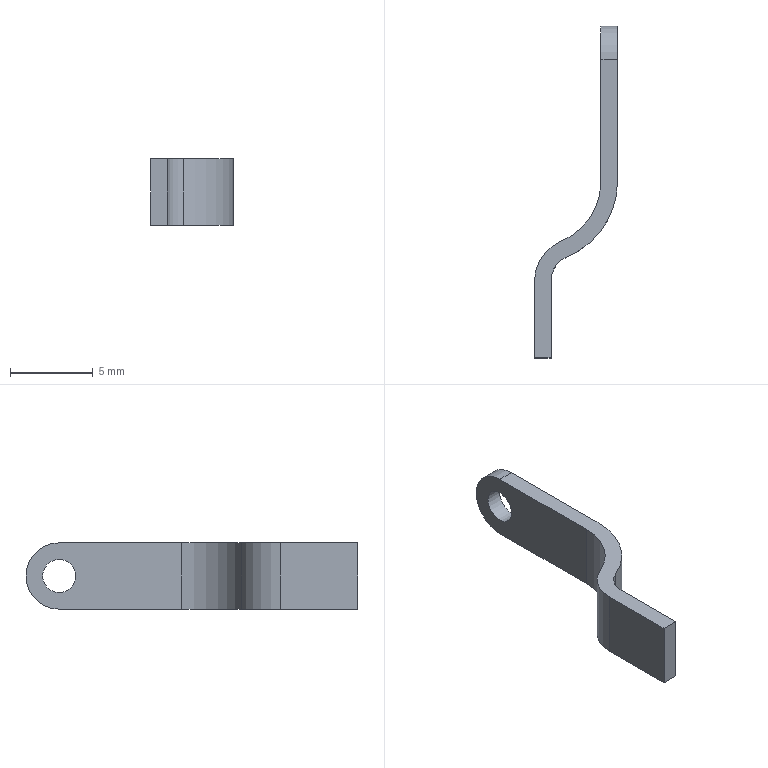Part | STEP file | 1-63.5 | 1 solid | 14 faces | box 5 x 20 x 4 mm | volume 81.74 mm3 | plane 7 | cylinder 7 | commonest cylinder face diameters 4 x2 2 x1 3.13 x1 5.13 x1 7.8 x1 9.8 x1
STEP:
#1=CARTESIAN_POINT('',(0.,0.,0.));
#2=DIRECTION('',(0.,0.,1.));
#3=DIRECTION('',(1.,0.,0.));
#4=AXIS2_PLACEMENT_3D('',#1,#2,#3);
#5=CARTESIAN_POINT('',(-4.,-15.,2.));
#6=VERTEX_POINT('',#5);
#7=CARTESIAN_POINT('',(-4.,-10.352,2.));
#8=VERTEX_POINT('',#7);
#9=CARTESIAN_POINT('',(-4.,-15.,2.));
#10=DIRECTION('',(0.,1.,0.));
#11=VECTOR('',#10,1.);
#12=LINE('',#9,#11);
#13=CARTESIAN_POINT('',(-4.,-12.676,0.));
#14=DIRECTION('',(-1.,0.,0.));
#15=DIRECTION('',(0.,1.,0.));
#16=AXIS2_PLACEMENT_3D('',#13,#14,#15);
#17=PLANE('',#16);
#18=CARTESIAN_POINT('',(-2.324,-2.));
#19=DIRECTION('',(1.,0.));
#20=VECTOR('',#19,1.);
#21=LINE('',#18,#20);
#22=(GEOMETRIC_REPRESENTATION_CONTEXT(2)PARAMETRIC_REPRESENTATION_CONTEXT()REPRESENTATION_CONTEXT('',''));
#23=DEFINITIONAL_REPRESENTATION('',(#21),#22);
#24=PCURVE('',#17,#23);
#25=CARTESIAN_POINT('',(-2.5,-5.,2.));
#26=DIRECTION('',(0.,0.,1.));
#27=DIRECTION('',(1.,0.,0.));
#28=AXIS2_PLACEMENT_3D('',#25,#26,#27);
#29=PLANE('',#28);
#30=CARTESIAN_POINT('',(-1.5,-10.));
#31=DIRECTION('',(0.,1.));
#32=VECTOR('',#31,1.);
#33=LINE('',#30,#32);
#34=(GEOMETRIC_REPRESENTATION_CONTEXT(2)PARAMETRIC_REPRESENTATION_CONTEXT()REPRESENTATION_CONTEXT('',''));
#35=DEFINITIONAL_REPRESENTATION('',(#33),#34);
#36=PCURVE('',#29,#35);
#37=SURFACE_CURVE('',#12,(#24,#36),.PCURVE_S1.);
#38=EDGE_CURVE('',#6,#8,#37,.T.);
#39=ORIENTED_EDGE('',*,*,#38,.T.);
#40=CARTESIAN_POINT('',(-4.,-10.352,-2.));
#41=VERTEX_POINT('',#40);
#42=CARTESIAN_POINT('',(-4.,-10.352,2.));
#43=DIRECTION('',(0.,0.,-1.));
#44=VECTOR('',#43,1.);
#45=LINE('',#42,#44);
#46=CARTESIAN_POINT('',(2.324,-2.));
#47=DIRECTION('',(0.,1.));
#48=VECTOR('',#47,1.);
#49=LINE('',#46,#48);
#50=(GEOMETRIC_REPRESENTATION_CONTEXT(2)PARAMETRIC_REPRESENTATION_CONTEXT()REPRESENTATION_CONTEXT('',''));
#51=DEFINITIONAL_REPRESENTATION('',(#49),#50);
#52=PCURVE('',#17,#51);
#53=CARTESIAN_POINT('',(-2.435,-10.352,2.));
#54=DIRECTION('',(0.,0.,-1.));
#55=DIRECTION('',(-1.,0.,0.));
#56=AXIS2_PLACEMENT_3D('',#53,#54,#55);
#57=CYLINDRICAL_SURFACE('',#56,1.565);
#58=CARTESIAN_POINT('',(0.,0.));
#59=DIRECTION('',(0.,1.));
#60=VECTOR('',#59,1.);
#61=LINE('',#58,#60);
#62=(GEOMETRIC_REPRESENTATION_CONTEXT(2)PARAMETRIC_REPRESENTATION_CONTEXT()REPRESENTATION_CONTEXT('',''));
#63=DEFINITIONAL_REPRESENTATION('',(#61),#62);
#64=PCURVE('',#57,#63);
#65=SURFACE_CURVE('',#45,(#52,#64),.PCURVE_S1.);
#66=EDGE_CURVE('',#8,#41,#65,.T.);
#67=ORIENTED_EDGE('',*,*,#66,.T.);
#68=CARTESIAN_POINT('',(-4.,-15.,-2.));
#69=VERTEX_POINT('',#68);
#70=CARTESIAN_POINT('',(-4.,-15.,-2.));
#71=DIRECTION('',(0.,1.,0.));
#72=VECTOR('',#71,1.);
#73=LINE('',#70,#72);
#74=CARTESIAN_POINT('',(-2.324,2.));
#75=DIRECTION('',(1.,0.));
#76=VECTOR('',#75,1.);
#77=LINE('',#74,#76);
#78=(GEOMETRIC_REPRESENTATION_CONTEXT(2)PARAMETRIC_REPRESENTATION_CONTEXT()REPRESENTATION_CONTEXT('',''));
#79=DEFINITIONAL_REPRESENTATION('',(#77),#78);
#80=PCURVE('',#17,#79);
#81=CARTESIAN_POINT('',(-2.5,-5.,-2.));
#82=DIRECTION('',(0.,0.,-1.));
#83=DIRECTION('',(-1.,0.,0.));
#84=AXIS2_PLACEMENT_3D('',#81,#82,#83);
#85=PLANE('',#84);
#86=CARTESIAN_POINT('',(1.5,-10.));
#87=DIRECTION('',(0.,1.));
#88=VECTOR('',#87,1.);
#89=LINE('',#86,#88);
#90=(GEOMETRIC_REPRESENTATION_CONTEXT(2)PARAMETRIC_REPRESENTATION_CONTEXT()REPRESENTATION_CONTEXT('',''));
#91=DEFINITIONAL_REPRESENTATION('',(#89),#90);
#92=PCURVE('',#85,#91);
#93=SURFACE_CURVE('',#73,(#80,#92),.PCURVE_S1.);
#94=EDGE_CURVE('',#69,#41,#93,.T.);
#95=ORIENTED_EDGE('',*,*,#94,.F.);
#96=CARTESIAN_POINT('',(-4.,-15.,2.));
#97=DIRECTION('',(0.,0.,-1.));
#98=VECTOR('',#97,1.);
#99=LINE('',#96,#98);
#100=CARTESIAN_POINT('',(-2.324,-2.));
#101=DIRECTION('',(0.,1.));
#102=VECTOR('',#101,1.);
#103=LINE('',#100,#102);
#104=(GEOMETRIC_REPRESENTATION_CONTEXT(2)PARAMETRIC_REPRESENTATION_CONTEXT()REPRESENTATION_CONTEXT('',''));
#105=DEFINITIONAL_REPRESENTATION('',(#103),#104);
#106=PCURVE('',#17,#105);
#107=CARTESIAN_POINT('',(-4.5,-15.,0.));
#108=DIRECTION('',(0.,1.,0.));
#109=DIRECTION('',(1.,0.,0.));
#110=AXIS2_PLACEMENT_3D('',#107,#108,#109);
#111=PLANE('',#110);
#112=CARTESIAN_POINT('',(0.5,-2.));
#113=DIRECTION('',(0.,1.));
#114=VECTOR('',#113,1.);
#115=LINE('',#112,#114);
#116=(GEOMETRIC_REPRESENTATION_CONTEXT(2)PARAMETRIC_REPRESENTATION_CONTEXT()REPRESENTATION_CONTEXT('',''));
#117=DEFINITIONAL_REPRESENTATION('',(#115),#116);
#118=PCURVE('',#111,#117);
#119=SURFACE_CURVE('',#99,(#106,#118),.PCURVE_S1.);
#120=EDGE_CURVE('',#6,#69,#119,.T.);
#121=ORIENTED_EDGE('',*,*,#120,.F.);
#122=EDGE_LOOP('',(#39,#67,#95,#121));
#123=FACE_BOUND('',#122,.F.);
#124=ADVANCED_FACE('',(#123),#17,.F.);
#125=CARTESIAN_POINT('',(-3.032,-8.905,2.));
#126=VERTEX_POINT('',#125);
#127=CARTESIAN_POINT('',(-2.435,-10.352,2.));
#128=DIRECTION('',(0.,0.,-1.));
#129=DIRECTION('',(-1.,0.,0.));
#130=AXIS2_PLACEMENT_3D('',#127,#128,#129);
#131=CIRCLE('',#130,1.565);
#132=CARTESIAN_POINT('',(0.,0.));
#133=DIRECTION('',(1.,0.));
#134=VECTOR('',#133,1.);
#135=LINE('',#132,#134);
#136=(GEOMETRIC_REPRESENTATION_CONTEXT(2)PARAMETRIC_REPRESENTATION_CONTEXT()REPRESENTATION_CONTEXT('',''));
#137=DEFINITIONAL_REPRESENTATION('',(#135),#136);
#138=PCURVE('',#57,#137);
#139=CARTESIAN_POINT('',(-1.5,-5.352));
#140=CARTESIAN_POINT('',(-1.5,-2.64));
#141=CARTESIAN_POINT('',(0.8479,-3.996));
#142=CARTESIAN_POINT('',(3.196,-5.352));
#143=CARTESIAN_POINT('',(0.8479,-6.707));
#144=CARTESIAN_POINT('',(-1.5,-8.063));
#145=CARTESIAN_POINT('',(-1.5,-5.352));
#146=(BOUNDED_CURVE()B_SPLINE_CURVE(2,(#139,#140,#141,#142,#143,#144,#145),.UNSPECIFIED.,.T.,.F.)B_SPLINE_CURVE_WITH_KNOTS((1,2,2,2,2,1),(-2.094,0.,2.094,4.189,6.283,8.378),.UNSPECIFIED.)CURVE()GEOMETRIC_REPRESENTATION_ITEM()RATIONAL_B_SPLINE_CURVE((1.,0.5,1.,0.5,1.,0.5,1.))REPRESENTATION_ITEM(''));
#147=(GEOMETRIC_REPRESENTATION_CONTEXT(2)PARAMETRIC_REPRESENTATION_CONTEXT()REPRESENTATION_CONTEXT('',''));
#148=DEFINITIONAL_REPRESENTATION('',(#146),#147);
#149=PCURVE('',#29,#148);
#150=SURFACE_CURVE('',#131,(#138,#149),.PCURVE_S1.);
#151=EDGE_CURVE('',#8,#126,#150,.T.);
#152=ORIENTED_EDGE('',*,*,#151,.T.);
#153=CARTESIAN_POINT('',(-3.032,-8.905,-2.));
#154=VERTEX_POINT('',#153);
#155=CARTESIAN_POINT('',(-3.032,-8.905,2.));
#156=DIRECTION('',(0.,0.,-1.));
#157=VECTOR('',#156,1.);
#158=LINE('',#155,#157);
#159=CARTESIAN_POINT('',(1.18,0.));
#160=DIRECTION('',(0.,1.));
#161=VECTOR('',#160,1.);
#162=LINE('',#159,#161);
#163=(GEOMETRIC_REPRESENTATION_CONTEXT(2)PARAMETRIC_REPRESENTATION_CONTEXT()REPRESENTATION_CONTEXT('',''));
#164=DEFINITIONAL_REPRESENTATION('',(#162),#163);
#165=PCURVE('',#57,#164);
#166=CARTESIAN_POINT('',(-4.9,-4.375,2.));
#167=DIRECTION('',(0.,0.,-1.));
#168=DIRECTION('',(0.3813,-0.9244,0.));
#169=AXIS2_PLACEMENT_3D('',#166,#167,#168);
#170=CYLINDRICAL_SURFACE('',#169,4.9);
#171=CARTESIAN_POINT('',(6.283,0.));
#172=DIRECTION('',(0.,1.));
#173=VECTOR('',#172,1.);
#174=LINE('',#171,#173);
#175=(GEOMETRIC_REPRESENTATION_CONTEXT(2)PARAMETRIC_REPRESENTATION_CONTEXT()REPRESENTATION_CONTEXT('',''));
#176=DEFINITIONAL_REPRESENTATION('',(#174),#175);
#177=PCURVE('',#170,#176);
#178=SURFACE_CURVE('',#158,(#165,#177),.PCURVE_S1.);
#179=EDGE_CURVE('',#126,#154,#178,.T.);
#180=ORIENTED_EDGE('',*,*,#179,.T.);
#181=CARTESIAN_POINT('',(-2.435,-10.352,-2.));
#182=DIRECTION('',(0.,0.,-1.));
#183=DIRECTION('',(-1.,0.,0.));
#184=AXIS2_PLACEMENT_3D('',#181,#182,#183);
#185=CIRCLE('',#184,1.565);
#186=CARTESIAN_POINT('',(0.,4.));
#187=DIRECTION('',(1.,0.));
#188=VECTOR('',#187,1.);
#189=LINE('',#186,#188);
#190=(GEOMETRIC_REPRESENTATION_CONTEXT(2)PARAMETRIC_REPRESENTATION_CONTEXT()REPRESENTATION_CONTEXT('',''));
#191=DEFINITIONAL_REPRESENTATION('',(#189),#190);
#192=PCURVE('',#57,#191);
#193=CARTESIAN_POINT('',(-0.06524,-5.352));
#194=DIRECTION('',(1.,0.));
#195=AXIS2_PLACEMENT_2D('',#193,#194);
#196=CIRCLE('',#195,1.565);
#197=(GEOMETRIC_REPRESENTATION_CONTEXT(2)PARAMETRIC_REPRESENTATION_CONTEXT()REPRESENTATION_CONTEXT('',''));
#198=DEFINITIONAL_REPRESENTATION('',(#196),#197);
#199=PCURVE('',#85,#198);
#200=SURFACE_CURVE('',#185,(#192,#199),.PCURVE_S1.);
#201=EDGE_CURVE('',#41,#154,#200,.T.);
#202=ORIENTED_EDGE('',*,*,#201,.F.);
#203=ORIENTED_EDGE('',*,*,#66,.F.);
#204=EDGE_LOOP('',(#152,#180,#202,#203));
#205=FACE_BOUND('',#204,.F.);
#206=ADVANCED_FACE('',(#205),#57,.F.);
#207=ORIENTED_EDGE('',*,*,#179,.T.);
#208=CARTESIAN_POINT('',(0.,-4.375,-2.));
#209=VERTEX_POINT('',#208);
#210=CARTESIAN_POINT('',(-4.9,-4.375,-2.));
#211=DIRECTION('',(0.,0.,1.));
#212=DIRECTION('',(0.3813,-0.9244,0.));
#213=AXIS2_PLACEMENT_3D('',#210,#211,#212);
#214=CIRCLE('',#213,4.9);
#215=CARTESIAN_POINT('',(6.283,4.));
#216=DIRECTION('',(-1.,0.));
#217=VECTOR('',#216,1.);
#218=LINE('',#215,#217);
#219=(GEOMETRIC_REPRESENTATION_CONTEXT(2)PARAMETRIC_REPRESENTATION_CONTEXT()REPRESENTATION_CONTEXT('',''));
#220=DEFINITIONAL_REPRESENTATION('',(#218),#219);
#221=PCURVE('',#170,#220);
#222=CARTESIAN_POINT('',(0.5316,-3.905));
#223=CARTESIAN_POINT('',(-7.314,-0.6681));
#224=CARTESIAN_POINT('',(-0.5886,4.509));
#225=CARTESIAN_POINT('',(6.137,9.685));
#226=CARTESIAN_POINT('',(7.258,1.272));
#227=CARTESIAN_POINT('',(8.378,-7.141));
#228=CARTESIAN_POINT('',(0.5316,-3.905));
#229=(BOUNDED_CURVE()B_SPLINE_CURVE(2,(#222,#223,#224,#225,#226,#227,#228),.UNSPECIFIED.,.T.,.F.)B_SPLINE_CURVE_WITH_KNOTS((1,2,2,2,2,1),(-2.094,0.,2.094,4.189,6.283,8.378),.UNSPECIFIED.)CURVE()GEOMETRIC_REPRESENTATION_ITEM()RATIONAL_B_SPLINE_CURVE((1.,0.5,1.,0.5,1.,0.5,1.))REPRESENTATION_ITEM(''));
#230=(GEOMETRIC_REPRESENTATION_CONTEXT(2)PARAMETRIC_REPRESENTATION_CONTEXT()REPRESENTATION_CONTEXT('',''));
#231=DEFINITIONAL_REPRESENTATION('',(#229),#230);
#232=PCURVE('',#85,#231);
#233=SURFACE_CURVE('',#214,(#221,#232),.PCURVE_S1.);
#234=EDGE_CURVE('',#154,#209,#233,.T.);
#235=ORIENTED_EDGE('',*,*,#234,.T.);
#236=CARTESIAN_POINT('',(0.,-4.375,2.));
#237=VERTEX_POINT('',#236);
#238=CARTESIAN_POINT('',(0.,-4.375,2.));
#239=DIRECTION('',(0.,0.,-1.));
#240=VECTOR('',#239,1.);
#241=LINE('',#238,#240);
#242=CARTESIAN_POINT('',(5.104,0.));
#243=DIRECTION('',(0.,1.));
#244=VECTOR('',#243,1.);
#245=LINE('',#242,#244);
#246=(GEOMETRIC_REPRESENTATION_CONTEXT(2)PARAMETRIC_REPRESENTATION_CONTEXT()REPRESENTATION_CONTEXT('',''));
#247=DEFINITIONAL_REPRESENTATION('',(#245),#246);
#248=PCURVE('',#170,#247);
#249=CARTESIAN_POINT('',(0.,1.672,0.08579));
#250=DIRECTION('',(-1.,0.,0.));
#251=DIRECTION('',(0.,1.,0.));
#252=AXIS2_PLACEMENT_3D('',#249,#250,#251);
#253=PLANE('',#252);
#254=CARTESIAN_POINT('',(-6.047,-1.914));
#255=DIRECTION('',(0.,1.));
#256=VECTOR('',#255,1.);
#257=LINE('',#254,#256);
#258=(GEOMETRIC_REPRESENTATION_CONTEXT(2)PARAMETRIC_REPRESENTATION_CONTEXT()REPRESENTATION_CONTEXT('',''));
#259=DEFINITIONAL_REPRESENTATION('',(#257),#258);
#260=PCURVE('',#253,#259);
#261=SURFACE_CURVE('',#241,(#248,#260),.PCURVE_S1.);
#262=EDGE_CURVE('',#237,#209,#261,.T.);
#263=ORIENTED_EDGE('',*,*,#262,.F.);
#264=CARTESIAN_POINT('',(-4.9,-4.375,2.));
#265=DIRECTION('',(0.,0.,1.));
#266=DIRECTION('',(0.3813,-0.9244,0.));
#267=AXIS2_PLACEMENT_3D('',#264,#265,#266);
#268=CIRCLE('',#267,4.9);
#269=CARTESIAN_POINT('',(6.283,0.));
#270=DIRECTION('',(-1.,0.));
#271=VECTOR('',#270,1.);
#272=LINE('',#269,#271);
#273=(GEOMETRIC_REPRESENTATION_CONTEXT(2)PARAMETRIC_REPRESENTATION_CONTEXT()REPRESENTATION_CONTEXT('',''));
#274=DEFINITIONAL_REPRESENTATION('',(#272),#273);
#275=PCURVE('',#170,#274);
#276=CARTESIAN_POINT('',(-2.4,0.6254));
#277=DIRECTION('',(0.3813,-0.9244));
#278=AXIS2_PLACEMENT_2D('',#276,#277);
#279=CIRCLE('',#278,4.9);
#280=(GEOMETRIC_REPRESENTATION_CONTEXT(2)PARAMETRIC_REPRESENTATION_CONTEXT()REPRESENTATION_CONTEXT('',''));
#281=DEFINITIONAL_REPRESENTATION('',(#279),#280);
#282=PCURVE('',#29,#281);
#283=SURFACE_CURVE('',#268,(#275,#282),.PCURVE_S1.);
#284=EDGE_CURVE('',#126,#237,#283,.T.);
#285=ORIENTED_EDGE('',*,*,#284,.F.);
#286=EDGE_LOOP('',(#207,#235,#263,#285));
#287=FACE_BOUND('',#286,.T.);
#288=ADVANCED_FACE('',(#287),#170,.T.);
#289=CARTESIAN_POINT('',(-5.,-15.,2.));
#290=VERTEX_POINT('',#289);
#291=CARTESIAN_POINT('',(-5.,-10.352,2.));
#292=VERTEX_POINT('',#291);
#293=CARTESIAN_POINT('',(-5.,-15.,2.));
#294=DIRECTION('',(0.,1.,0.));
#295=VECTOR('',#294,1.);
#296=LINE('',#293,#295);
#297=CARTESIAN_POINT('',(-5.,-12.676,0.));
#298=DIRECTION('',(-1.,0.,0.));
#299=DIRECTION('',(0.,1.,0.));
#300=AXIS2_PLACEMENT_3D('',#297,#298,#299);
#301=PLANE('',#300);
#302=CARTESIAN_POINT('',(-2.324,-2.));
#303=DIRECTION('',(1.,0.));
#304=VECTOR('',#303,1.);
#305=LINE('',#302,#304);
#306=(GEOMETRIC_REPRESENTATION_CONTEXT(2)PARAMETRIC_REPRESENTATION_CONTEXT()REPRESENTATION_CONTEXT('',''));
#307=DEFINITIONAL_REPRESENTATION('',(#305),#306);
#308=PCURVE('',#301,#307);
#309=CARTESIAN_POINT('',(-2.5,-10.));
#310=DIRECTION('',(0.,1.));
#311=VECTOR('',#310,1.);
#312=LINE('',#309,#311);
#313=(GEOMETRIC_REPRESENTATION_CONTEXT(2)PARAMETRIC_REPRESENTATION_CONTEXT()REPRESENTATION_CONTEXT('',''));
#314=DEFINITIONAL_REPRESENTATION('',(#312),#313);
#315=PCURVE('',#29,#314);
#316=SURFACE_CURVE('',#296,(#308,#315),.PCURVE_S1.);
#317=EDGE_CURVE('',#290,#292,#316,.T.);
#318=ORIENTED_EDGE('',*,*,#317,.T.);
#319=CARTESIAN_POINT('',(-5.,-10.352,-2.));
#320=VERTEX_POINT('',#319);
#321=CARTESIAN_POINT('',(-5.,-10.352,2.));
#322=DIRECTION('',(0.,0.,-1.));
#323=VECTOR('',#322,1.);
#324=LINE('',#321,#323);
#325=CARTESIAN_POINT('',(2.324,-2.));
#326=DIRECTION('',(0.,1.));
#327=VECTOR('',#326,1.);
#328=LINE('',#325,#327);
#329=(GEOMETRIC_REPRESENTATION_CONTEXT(2)PARAMETRIC_REPRESENTATION_CONTEXT()REPRESENTATION_CONTEXT('',''));
#330=DEFINITIONAL_REPRESENTATION('',(#328),#329);
#331=PCURVE('',#301,#330);
#332=CARTESIAN_POINT('',(-2.435,-10.352,2.));
#333=DIRECTION('',(0.,0.,-1.));
#334=DIRECTION('',(-1.,0.,0.));
#335=AXIS2_PLACEMENT_3D('',#332,#333,#334);
#336=CYLINDRICAL_SURFACE('',#335,2.565);
#337=CARTESIAN_POINT('',(0.,0.));
#338=DIRECTION('',(0.,1.));
#339=VECTOR('',#338,1.);
#340=LINE('',#337,#339);
#341=(GEOMETRIC_REPRESENTATION_CONTEXT(2)PARAMETRIC_REPRESENTATION_CONTEXT()REPRESENTATION_CONTEXT('',''));
#342=DEFINITIONAL_REPRESENTATION('',(#340),#341);
#343=PCURVE('',#336,#342);
#344=SURFACE_CURVE('',#324,(#331,#343),.PCURVE_S1.);
#345=EDGE_CURVE('',#292,#320,#344,.T.);
#346=ORIENTED_EDGE('',*,*,#345,.T.);
#347=CARTESIAN_POINT('',(-5.,-15.,-2.));
#348=VERTEX_POINT('',#347);
#349=CARTESIAN_POINT('',(-5.,-10.352,-2.));
#350=DIRECTION('',(0.,-1.,0.));
#351=VECTOR('',#350,1.);
#352=LINE('',#349,#351);
#353=CARTESIAN_POINT('',(2.324,2.));
#354=DIRECTION('',(-1.,0.));
#355=VECTOR('',#354,1.);
#356=LINE('',#353,#355);
#357=(GEOMETRIC_REPRESENTATION_CONTEXT(2)PARAMETRIC_REPRESENTATION_CONTEXT()REPRESENTATION_CONTEXT('',''));
#358=DEFINITIONAL_REPRESENTATION('',(#356),#357);
#359=PCURVE('',#301,#358);
#360=CARTESIAN_POINT('',(2.5,-5.352));
#361=DIRECTION('',(0.,-1.));
#362=VECTOR('',#361,1.);
#363=LINE('',#360,#362);
#364=(GEOMETRIC_REPRESENTATION_CONTEXT(2)PARAMETRIC_REPRESENTATION_CONTEXT()REPRESENTATION_CONTEXT('',''));
#365=DEFINITIONAL_REPRESENTATION('',(#363),#364);
#366=PCURVE('',#85,#365);
#367=SURFACE_CURVE('',#352,(#359,#366),.PCURVE_S1.);
#368=EDGE_CURVE('',#320,#348,#367,.T.);
#369=ORIENTED_EDGE('',*,*,#368,.T.);
#370=CARTESIAN_POINT('',(-5.,-15.,-2.));
#371=DIRECTION('',(0.,0.,1.));
#372=VECTOR('',#371,1.);
#373=LINE('',#370,#372);
#374=CARTESIAN_POINT('',(-2.324,2.));
#375=DIRECTION('',(0.,-1.));
#376=VECTOR('',#375,1.);
#377=LINE('',#374,#376);
#378=(GEOMETRIC_REPRESENTATION_CONTEXT(2)PARAMETRIC_REPRESENTATION_CONTEXT()REPRESENTATION_CONTEXT('',''));
#379=DEFINITIONAL_REPRESENTATION('',(#377),#378);
#380=PCURVE('',#301,#379);
#381=CARTESIAN_POINT('',(-0.5,2.));
#382=DIRECTION('',(0.,-1.));
#383=VECTOR('',#382,1.);
#384=LINE('',#381,#383);
#385=(GEOMETRIC_REPRESENTATION_CONTEXT(2)PARAMETRIC_REPRESENTATION_CONTEXT()REPRESENTATION_CONTEXT('',''));
#386=DEFINITIONAL_REPRESENTATION('',(#384),#385);
#387=PCURVE('',#111,#386);
#388=SURFACE_CURVE('',#373,(#380,#387),.PCURVE_S1.);
#389=EDGE_CURVE('',#348,#290,#388,.T.);
#390=ORIENTED_EDGE('',*,*,#389,.T.);
#391=EDGE_LOOP('',(#318,#346,#369,#390));
#392=FACE_BOUND('',#391,.T.);
#393=ADVANCED_FACE('',(#392),#301,.T.);
#394=CARTESIAN_POINT('',(-3.413,-7.98,2.));
#395=VERTEX_POINT('',#394);
#396=CARTESIAN_POINT('',(-2.435,-10.352,2.));
#397=DIRECTION('',(0.,0.,-1.));
#398=DIRECTION('',(-1.,0.,0.));
#399=AXIS2_PLACEMENT_3D('',#396,#397,#398);
#400=CIRCLE('',#399,2.565);
#401=CARTESIAN_POINT('',(0.,0.));
#402=DIRECTION('',(1.,0.));
#403=VECTOR('',#402,1.);
#404=LINE('',#401,#403);
#405=(GEOMETRIC_REPRESENTATION_CONTEXT(2)PARAMETRIC_REPRESENTATION_CONTEXT()REPRESENTATION_CONTEXT('',''));
#406=DEFINITIONAL_REPRESENTATION('',(#404),#405);
#407=PCURVE('',#336,#406);
#408=CARTESIAN_POINT('',(-2.5,-5.352));
#409=CARTESIAN_POINT('',(-2.5,-0.9084));
#410=CARTESIAN_POINT('',(1.348,-3.13));
#411=CARTESIAN_POINT('',(5.196,-5.352));
#412=CARTESIAN_POINT('',(1.348,-7.573));
#413=CARTESIAN_POINT('',(-2.5,-9.795));
#414=CARTESIAN_POINT('',(-2.5,-5.352));
#415=(BOUNDED_CURVE()B_SPLINE_CURVE(2,(#408,#409,#410,#411,#412,#413,#414),.UNSPECIFIED.,.T.,.F.)B_SPLINE_CURVE_WITH_KNOTS((1,2,2,2,2,1),(-2.094,0.,2.094,4.189,6.283,8.378),.UNSPECIFIED.)CURVE()GEOMETRIC_REPRESENTATION_ITEM()RATIONAL_B_SPLINE_CURVE((1.,0.5,1.,0.5,1.,0.5,1.))REPRESENTATION_ITEM(''));
#416=(GEOMETRIC_REPRESENTATION_CONTEXT(2)PARAMETRIC_REPRESENTATION_CONTEXT()REPRESENTATION_CONTEXT('',''));
#417=DEFINITIONAL_REPRESENTATION('',(#415),#416);
#418=PCURVE('',#29,#417);
#419=SURFACE_CURVE('',#400,(#407,#418),.PCURVE_S1.);
#420=EDGE_CURVE('',#292,#395,#419,.T.);
#421=ORIENTED_EDGE('',*,*,#420,.T.);
#422=CARTESIAN_POINT('',(-3.413,-7.98,-2.));
#423=VERTEX_POINT('',#422);
#424=CARTESIAN_POINT('',(-3.413,-7.98,2.));
#425=DIRECTION('',(0.,0.,-1.));
#426=VECTOR('',#425,1.);
#427=LINE('',#424,#426);
#428=CARTESIAN_POINT('',(1.18,0.));
#429=DIRECTION('',(0.,1.));
#430=VECTOR('',#429,1.);
#431=LINE('',#428,#430);
#432=(GEOMETRIC_REPRESENTATION_CONTEXT(2)PARAMETRIC_REPRESENTATION_CONTEXT()REPRESENTATION_CONTEXT('',''));
#433=DEFINITIONAL_REPRESENTATION('',(#431),#432);
#434=PCURVE('',#336,#433);
#435=CARTESIAN_POINT('',(-4.9,-4.375,2.));
#436=DIRECTION('',(0.,0.,-1.));
#437=DIRECTION('',(0.3813,-0.9244,0.));
#438=AXIS2_PLACEMENT_3D('',#435,#436,#437);
#439=CYLINDRICAL_SURFACE('',#438,3.9);
#440=CARTESIAN_POINT('',(6.283,0.));
#441=DIRECTION('',(0.,1.));
#442=VECTOR('',#441,1.);
#443=LINE('',#440,#442);
#444=(GEOMETRIC_REPRESENTATION_CONTEXT(2)PARAMETRIC_REPRESENTATION_CONTEXT()REPRESENTATION_CONTEXT('',''));
#445=DEFINITIONAL_REPRESENTATION('',(#443),#444);
#446=PCURVE('',#439,#445);
#447=SURFACE_CURVE('',#427,(#434,#446),.PCURVE_S1.);
#448=EDGE_CURVE('',#395,#423,#447,.T.);
#449=ORIENTED_EDGE('',*,*,#448,.T.);
#450=CARTESIAN_POINT('',(-2.435,-10.352,-2.));
#451=DIRECTION('',(0.,0.,1.));
#452=DIRECTION('',(-0.3813,0.9244,0.));
#453=AXIS2_PLACEMENT_3D('',#450,#451,#452);
#454=CIRCLE('',#453,2.565);
#455=CARTESIAN_POINT('',(1.18,4.));
#456=DIRECTION('',(-1.,0.));
#457=VECTOR('',#456,1.);
#458=LINE('',#455,#457);
#459=(GEOMETRIC_REPRESENTATION_CONTEXT(2)PARAMETRIC_REPRESENTATION_CONTEXT()REPRESENTATION_CONTEXT('',''));
#460=DEFINITIONAL_REPRESENTATION('',(#458),#459);
#461=PCURVE('',#336,#460);
#462=CARTESIAN_POINT('',(0.913,-2.98));
#463=CARTESIAN_POINT('',(5.02,-4.674));
#464=CARTESIAN_POINT('',(1.499,-7.384));
#465=CARTESIAN_POINT('',(-2.022,-10.094));
#466=CARTESIAN_POINT('',(-2.608,-5.69));
#467=CARTESIAN_POINT('',(-3.194,-1.286));
#468=CARTESIAN_POINT('',(0.913,-2.98));
#469=(BOUNDED_CURVE()B_SPLINE_CURVE(2,(#462,#463,#464,#465,#466,#467,#468),.UNSPECIFIED.,.T.,.F.)B_SPLINE_CURVE_WITH_KNOTS((1,2,2,2,2,1),(-2.094,0.,2.094,4.189,6.283,8.378),.UNSPECIFIED.)CURVE()GEOMETRIC_REPRESENTATION_ITEM()RATIONAL_B_SPLINE_CURVE((1.,0.5,1.,0.5,1.,0.5,1.))REPRESENTATION_ITEM(''));
#470=(GEOMETRIC_REPRESENTATION_CONTEXT(2)PARAMETRIC_REPRESENTATION_CONTEXT()REPRESENTATION_CONTEXT('',''));
#471=DEFINITIONAL_REPRESENTATION('',(#469),#470);
#472=PCURVE('',#85,#471);
#473=SURFACE_CURVE('',#454,(#461,#472),.PCURVE_S1.);
#474=EDGE_CURVE('',#423,#320,#473,.T.);
#475=ORIENTED_EDGE('',*,*,#474,.T.);
#476=ORIENTED_EDGE('',*,*,#345,.F.);
#477=EDGE_LOOP('',(#421,#449,#475,#476));
#478=FACE_BOUND('',#477,.T.);
#479=ADVANCED_FACE('',(#478),#336,.T.);
#480=ORIENTED_EDGE('',*,*,#448,.T.);
#481=CARTESIAN_POINT('',(-1.,-4.375,-2.));
#482=VERTEX_POINT('',#481);
#483=CARTESIAN_POINT('',(-4.9,-4.375,-2.));
#484=DIRECTION('',(0.,0.,-1.));
#485=DIRECTION('',(1.,0.,0.));
#486=AXIS2_PLACEMENT_3D('',#483,#484,#485);
#487=CIRCLE('',#486,3.9);
#488=CARTESIAN_POINT('',(5.104,4.));
#489=DIRECTION('',(1.,0.));
#490=VECTOR('',#489,1.);
#491=LINE('',#488,#490);
#492=(GEOMETRIC_REPRESENTATION_CONTEXT(2)PARAMETRIC_REPRESENTATION_CONTEXT()REPRESENTATION_CONTEXT('',''));
#493=DEFINITIONAL_REPRESENTATION('',(#491),#492);
#494=PCURVE('',#439,#493);
#495=CARTESIAN_POINT('',(2.4,0.6254));
#496=DIRECTION('',(-1.,0.));
#497=AXIS2_PLACEMENT_2D('',#495,#496);
#498=CIRCLE('',#497,3.9);
#499=(GEOMETRIC_REPRESENTATION_CONTEXT(2)PARAMETRIC_REPRESENTATION_CONTEXT()REPRESENTATION_CONTEXT('',''));
#500=DEFINITIONAL_REPRESENTATION('',(#498),#499);
#501=PCURVE('',#85,#500);
#502=SURFACE_CURVE('',#487,(#494,#501),.PCURVE_S1.);
#503=EDGE_CURVE('',#482,#423,#502,.T.);
#504=ORIENTED_EDGE('',*,*,#503,.F.);
#505=CARTESIAN_POINT('',(-1.,-4.375,2.));
#506=VERTEX_POINT('',#505);
#507=CARTESIAN_POINT('',(-1.,-4.375,2.));
#508=DIRECTION('',(0.,0.,-1.));
#509=VECTOR('',#508,1.);
#510=LINE('',#507,#509);
#511=CARTESIAN_POINT('',(5.104,0.));
#512=DIRECTION('',(0.,1.));
#513=VECTOR('',#512,1.);
#514=LINE('',#511,#513);
#515=(GEOMETRIC_REPRESENTATION_CONTEXT(2)PARAMETRIC_REPRESENTATION_CONTEXT()REPRESENTATION_CONTEXT('',''));
#516=DEFINITIONAL_REPRESENTATION('',(#514),#515);
#517=PCURVE('',#439,#516);
#518=CARTESIAN_POINT('',(-1.,3.354,0.));
#519=DIRECTION('',(-1.,0.,0.));
#520=DIRECTION('',(0.,1.,0.));
#521=AXIS2_PLACEMENT_3D('',#518,#519,#520);
#522=PLANE('',#521);
#523=CARTESIAN_POINT('',(-7.729,-2.));
#524=DIRECTION('',(0.,1.));
#525=VECTOR('',#524,1.);
#526=LINE('',#523,#525);
#527=(GEOMETRIC_REPRESENTATION_CONTEXT(2)PARAMETRIC_REPRESENTATION_CONTEXT()REPRESENTATION_CONTEXT('',''));
#528=DEFINITIONAL_REPRESENTATION('',(#526),#527);
#529=PCURVE('',#522,#528);
#530=SURFACE_CURVE('',#510,(#517,#529),.PCURVE_S1.);
#531=EDGE_CURVE('',#506,#482,#530,.T.);
#532=ORIENTED_EDGE('',*,*,#531,.F.);
#533=CARTESIAN_POINT('',(-4.9,-4.375,2.));
#534=DIRECTION('',(0.,0.,1.));
#535=DIRECTION('',(0.3813,-0.9244,0.));
#536=AXIS2_PLACEMENT_3D('',#533,#534,#535);
#537=CIRCLE('',#536,3.9);
#538=CARTESIAN_POINT('',(6.283,0.));
#539=DIRECTION('',(-1.,0.));
#540=VECTOR('',#539,1.);
#541=LINE('',#538,#540);
#542=(GEOMETRIC_REPRESENTATION_CONTEXT(2)PARAMETRIC_REPRESENTATION_CONTEXT()REPRESENTATION_CONTEXT('',''));
#543=DEFINITIONAL_REPRESENTATION('',(#541),#542);
#544=PCURVE('',#439,#543);
#545=CARTESIAN_POINT('',(-2.4,0.6254));
#546=DIRECTION('',(0.3813,-0.9244));
#547=AXIS2_PLACEMENT_2D('',#545,#546);
#548=CIRCLE('',#547,3.9);
#549=(GEOMETRIC_REPRESENTATION_CONTEXT(2)PARAMETRIC_REPRESENTATION_CONTEXT()REPRESENTATION_CONTEXT('',''));
#550=DEFINITIONAL_REPRESENTATION('',(#548),#549);
#551=PCURVE('',#29,#550);
#552=SURFACE_CURVE('',#537,(#544,#551),.PCURVE_S1.);
#553=EDGE_CURVE('',#395,#506,#552,.T.);
#554=ORIENTED_EDGE('',*,*,#553,.F.);
#555=EDGE_LOOP('',(#480,#504,#532,#554));
#556=FACE_BOUND('',#555,.F.);
#557=ADVANCED_FACE('',(#556),#439,.F.);
#558=ORIENTED_EDGE('',*,*,#120,.T.);
#559=CARTESIAN_POINT('',(-5.,-15.,-2.));
#560=DIRECTION('',(1.,0.,0.));
#561=VECTOR('',#560,1.);
#562=LINE('',#559,#561);
#563=CARTESIAN_POINT('',(-0.5,2.));
#564=DIRECTION('',(1.,0.));
#565=VECTOR('',#564,1.);
#566=LINE('',#563,#565);
#567=(GEOMETRIC_REPRESENTATION_CONTEXT(2)PARAMETRIC_REPRESENTATION_CONTEXT()REPRESENTATION_CONTEXT('',''));
#568=DEFINITIONAL_REPRESENTATION('',(#566),#567);
#569=PCURVE('',#111,#568);
#570=CARTESIAN_POINT('',(2.5,-10.));
#571=DIRECTION('',(-1.,0.));
#572=VECTOR('',#571,1.);
#573=LINE('',#570,#572);
#574=(GEOMETRIC_REPRESENTATION_CONTEXT(2)PARAMETRIC_REPRESENTATION_CONTEXT()REPRESENTATION_CONTEXT('',''));
#575=DEFINITIONAL_REPRESENTATION('',(#573),#574);
#576=PCURVE('',#85,#575);
#577=SURFACE_CURVE('',#562,(#569,#576),.PCURVE_S1.);
#578=EDGE_CURVE('',#348,#69,#577,.T.);
#579=ORIENTED_EDGE('',*,*,#578,.F.);
#580=ORIENTED_EDGE('',*,*,#389,.T.);
#581=CARTESIAN_POINT('',(-5.,-15.,2.));
#582=DIRECTION('',(1.,0.,0.));
#583=VECTOR('',#582,1.);
#584=LINE('',#581,#583);
#585=CARTESIAN_POINT('',(-0.5,-2.));
#586=DIRECTION('',(1.,0.));
#587=VECTOR('',#586,1.);
#588=LINE('',#585,#587);
#589=(GEOMETRIC_REPRESENTATION_CONTEXT(2)PARAMETRIC_REPRESENTATION_CONTEXT()REPRESENTATION_CONTEXT('',''));
#590=DEFINITIONAL_REPRESENTATION('',(#588),#589);
#591=PCURVE('',#111,#590);
#592=CARTESIAN_POINT('',(-2.5,-10.));
#593=DIRECTION('',(1.,0.));
#594=VECTOR('',#593,1.);
#595=LINE('',#592,#594);
#596=(GEOMETRIC_REPRESENTATION_CONTEXT(2)PARAMETRIC_REPRESENTATION_CONTEXT()REPRESENTATION_CONTEXT('',''));
#597=DEFINITIONAL_REPRESENTATION('',(#595),#596);
#598=PCURVE('',#29,#597);
#599=SURFACE_CURVE('',#584,(#591,#598),.PCURVE_S1.);
#600=EDGE_CURVE('',#290,#6,#599,.T.);
#601=ORIENTED_EDGE('',*,*,#600,.T.);
#602=EDGE_LOOP('',(#558,#579,#580,#601));
#603=FACE_BOUND('',#602,.F.);
#604=ADVANCED_FACE('',(#603),#111,.F.);
#605=CARTESIAN_POINT('',(0.,4.,0.));
#606=VERTEX_POINT('',#605);
#607=CARTESIAN_POINT('',(0.,3.,0.));
#608=DIRECTION('',(1.,0.,0.));
#609=DIRECTION('',(0.,1.,0.));
#610=AXIS2_PLACEMENT_3D('',#607,#608,#609);
#611=CIRCLE('',#610,1.);
#612=CARTESIAN_POINT('',(15.,3.,0.));
#613=DIRECTION('',(-1.,0.,0.));
#614=DIRECTION('',(0.,1.,0.));
#615=AXIS2_PLACEMENT_3D('',#612,#613,#614);
#616=CYLINDRICAL_SURFACE('',#615,1.);
#617=CARTESIAN_POINT('',(6.283,15.));
#618=DIRECTION('',(-1.,0.));
#619=VECTOR('',#618,1.);
#620=LINE('',#617,#619);
#621=(GEOMETRIC_REPRESENTATION_CONTEXT(2)PARAMETRIC_REPRESENTATION_CONTEXT()REPRESENTATION_CONTEXT('',''));
#622=DEFINITIONAL_REPRESENTATION('',(#620),#621);
#623=PCURVE('',#616,#622);
#624=CARTESIAN_POINT('',(2.328,0.08579));
#625=CARTESIAN_POINT('',(2.328,-1.646));
#626=CARTESIAN_POINT('',(0.8279,-0.7802));
#627=CARTESIAN_POINT('',(-0.6721,0.08579));
#628=CARTESIAN_POINT('',(0.8279,0.9518));
#629=CARTESIAN_POINT('',(2.328,1.818));
#630=CARTESIAN_POINT('',(2.328,0.08579));
#631=(BOUNDED_CURVE()B_SPLINE_CURVE(2,(#624,#625,#626,#627,#628,#629,#630),.UNSPECIFIED.,.T.,.F.)B_SPLINE_CURVE_WITH_KNOTS((1,2,2,2,2,1),(-2.094,0.,2.094,4.189,6.283,8.378),.UNSPECIFIED.)CURVE()GEOMETRIC_REPRESENTATION_ITEM()RATIONAL_B_SPLINE_CURVE((1.,0.5,1.,0.5,1.,0.5,1.))REPRESENTATION_ITEM(''));
#632=(GEOMETRIC_REPRESENTATION_CONTEXT(2)PARAMETRIC_REPRESENTATION_CONTEXT()REPRESENTATION_CONTEXT('',''));
#633=DEFINITIONAL_REPRESENTATION('',(#631),#632);
#634=PCURVE('',#253,#633);
#635=SURFACE_CURVE('',#611,(#623,#634),.PCURVE_S1.);
#636=EDGE_CURVE('',#606,#606,#635,.T.);
#637=ORIENTED_EDGE('',*,*,#636,.F.);
#638=CARTESIAN_POINT('',(-1.,4.,0.));
#639=VERTEX_POINT('',#638);
#640=CARTESIAN_POINT('',(0.,4.,0.));
#641=DIRECTION('',(-1.,0.,0.));
#642=VECTOR('',#641,1.);
#643=LINE('',#640,#642);
#644=CARTESIAN_POINT('',(6.283,15.));
#645=DIRECTION('',(0.,1.));
#646=VECTOR('',#645,1.);
#647=LINE('',#644,#646);
#648=(GEOMETRIC_REPRESENTATION_CONTEXT(2)PARAMETRIC_REPRESENTATION_CONTEXT()REPRESENTATION_CONTEXT('',''));
#649=DEFINITIONAL_REPRESENTATION('',(#647),#648);
#650=PCURVE('',#616,#649);
#651=CARTESIAN_POINT('',(0.,15.));
#652=DIRECTION('',(0.,1.));
#653=VECTOR('',#652,1.);
#654=LINE('',#651,#653);
#655=(GEOMETRIC_REPRESENTATION_CONTEXT(2)PARAMETRIC_REPRESENTATION_CONTEXT()REPRESENTATION_CONTEXT('',''));
#656=DEFINITIONAL_REPRESENTATION('',(#654),#655);
#657=PCURVE('',#616,#656);
#658=SEAM_CURVE('',#643,(#650,#657),.PCURVE_S1.);
#659=EDGE_CURVE('',#606,#639,#658,.T.);
#660=ORIENTED_EDGE('',*,*,#659,.T.);
#661=CARTESIAN_POINT('',(-1.,3.,0.));
#662=DIRECTION('',(-1.,0.,0.));
#663=DIRECTION('',(0.,1.,0.));
#664=AXIS2_PLACEMENT_3D('',#661,#662,#663);
#665=CIRCLE('',#664,1.);
#666=CARTESIAN_POINT('',(0.,16.));
#667=DIRECTION('',(1.,0.));
#668=VECTOR('',#667,1.);
#669=LINE('',#666,#668);
#670=(GEOMETRIC_REPRESENTATION_CONTEXT(2)PARAMETRIC_REPRESENTATION_CONTEXT()REPRESENTATION_CONTEXT('',''));
#671=DEFINITIONAL_REPRESENTATION('',(#669),#670);
#672=PCURVE('',#616,#671);
#673=CARTESIAN_POINT('',(-0.3541,0.));
#674=DIRECTION('',(1.,0.));
#675=AXIS2_PLACEMENT_2D('',#673,#674);
#676=CIRCLE('',#675,1.);
#677=(GEOMETRIC_REPRESENTATION_CONTEXT(2)PARAMETRIC_REPRESENTATION_CONTEXT()REPRESENTATION_CONTEXT('',''));
#678=DEFINITIONAL_REPRESENTATION('',(#676),#677);
#679=PCURVE('',#522,#678);
#680=SURFACE_CURVE('',#665,(#672,#679),.PCURVE_S1.);
#681=EDGE_CURVE('',#639,#639,#680,.T.);
#682=ORIENTED_EDGE('',*,*,#681,.F.);
#683=ORIENTED_EDGE('',*,*,#659,.F.);
#684=EDGE_LOOP('',(#637,#660,#682,#683));
#685=FACE_BOUND('',#684,.F.);
#686=ADVANCED_FACE('',(#685),#616,.F.);
#687=ORIENTED_EDGE('',*,*,#553,.F.);
#688=ORIENTED_EDGE('',*,*,#420,.F.);
#689=ORIENTED_EDGE('',*,*,#317,.F.);
#690=ORIENTED_EDGE('',*,*,#600,.T.);
#691=ORIENTED_EDGE('',*,*,#38,.T.);
#692=ORIENTED_EDGE('',*,*,#151,.T.);
#693=ORIENTED_EDGE('',*,*,#284,.T.);
#694=CARTESIAN_POINT('',(0.,3.,2.));
#695=VERTEX_POINT('',#694);
#696=CARTESIAN_POINT('',(0.,-4.375,2.));
#697=DIRECTION('',(0.,1.,0.));
#698=VECTOR('',#697,1.);
#699=LINE('',#696,#698);
#700=CARTESIAN_POINT('',(2.5,0.6254));
#701=DIRECTION('',(0.,1.));
#702=VECTOR('',#701,1.);
#703=LINE('',#700,#702);
#704=(GEOMETRIC_REPRESENTATION_CONTEXT(2)PARAMETRIC_REPRESENTATION_CONTEXT()REPRESENTATION_CONTEXT('',''));
#705=DEFINITIONAL_REPRESENTATION('',(#703),#704);
#706=PCURVE('',#29,#705);
#707=CARTESIAN_POINT('',(-6.047,-1.914));
#708=DIRECTION('',(1.,0.));
#709=VECTOR('',#708,1.);
#710=LINE('',#707,#709);
#711=(GEOMETRIC_REPRESENTATION_CONTEXT(2)PARAMETRIC_REPRESENTATION_CONTEXT()REPRESENTATION_CONTEXT('',''));
#712=DEFINITIONAL_REPRESENTATION('',(#710),#711);
#713=PCURVE('',#253,#712);
#714=SURFACE_CURVE('',#699,(#706,#713),.PCURVE_S1.);
#715=EDGE_CURVE('',#237,#695,#714,.T.);
#716=ORIENTED_EDGE('',*,*,#715,.T.);
#717=CARTESIAN_POINT('',(-1.,3.,2.));
#718=VERTEX_POINT('',#717);
#719=CARTESIAN_POINT('',(0.,3.,2.));
#720=DIRECTION('',(-1.,0.,0.));
#721=VECTOR('',#720,1.);
#722=LINE('',#719,#721);
#723=CARTESIAN_POINT('',(2.5,8.));
#724=DIRECTION('',(-1.,0.));
#725=VECTOR('',#724,1.);
#726=LINE('',#723,#725);
#727=(GEOMETRIC_REPRESENTATION_CONTEXT(2)PARAMETRIC_REPRESENTATION_CONTEXT()REPRESENTATION_CONTEXT('',''));
#728=DEFINITIONAL_REPRESENTATION('',(#726),#727);
#729=PCURVE('',#29,#728);
#730=CARTESIAN_POINT('',(2.978,3.,0.));
#731=DIRECTION('',(-1.,0.,0.));
#732=DIRECTION('',(0.,0.,1.));
#733=AXIS2_PLACEMENT_3D('',#730,#731,#732);
#734=CYLINDRICAL_SURFACE('',#733,2.);
#735=CARTESIAN_POINT('',(0.,2.978));
#736=DIRECTION('',(0.,1.));
#737=VECTOR('',#736,1.);
#738=LINE('',#735,#737);
#739=(GEOMETRIC_REPRESENTATION_CONTEXT(2)PARAMETRIC_REPRESENTATION_CONTEXT()REPRESENTATION_CONTEXT('',''));
#740=DEFINITIONAL_REPRESENTATION('',(#738),#739);
#741=PCURVE('',#734,#740);
#742=SURFACE_CURVE('',#722,(#729,#741),.PCURVE_S1.);
#743=EDGE_CURVE('',#695,#718,#742,.T.);
#744=ORIENTED_EDGE('',*,*,#743,.T.);
#745=CARTESIAN_POINT('',(-1.,-4.375,2.));
#746=DIRECTION('',(0.,1.,0.));
#747=VECTOR('',#746,1.);
#748=LINE('',#745,#747);
#749=CARTESIAN_POINT('',(1.5,0.6254));
#750=DIRECTION('',(0.,1.));
#751=VECTOR('',#750,1.);
#752=LINE('',#749,#751);
#753=(GEOMETRIC_REPRESENTATION_CONTEXT(2)PARAMETRIC_REPRESENTATION_CONTEXT()REPRESENTATION_CONTEXT('',''));
#754=DEFINITIONAL_REPRESENTATION('',(#752),#753);
#755=PCURVE('',#29,#754);
#756=CARTESIAN_POINT('',(-7.729,-2.));
#757=DIRECTION('',(1.,0.));
#758=VECTOR('',#757,1.);
#759=LINE('',#756,#758);
#760=(GEOMETRIC_REPRESENTATION_CONTEXT(2)PARAMETRIC_REPRESENTATION_CONTEXT()REPRESENTATION_CONTEXT('',''));
#761=DEFINITIONAL_REPRESENTATION('',(#759),#760);
#762=PCURVE('',#522,#761);
#763=SURFACE_CURVE('',#748,(#755,#762),.PCURVE_S1.);
#764=EDGE_CURVE('',#506,#718,#763,.T.);
#765=ORIENTED_EDGE('',*,*,#764,.F.);
#766=EDGE_LOOP('',(#687,#688,#689,#690,#691,#692,#693,#716,#744,#765));
#767=FACE_BOUND('',#766,.T.);
#768=ADVANCED_FACE('',(#767),#29,.T.);
#769=ORIENTED_EDGE('',*,*,#234,.F.);
#770=ORIENTED_EDGE('',*,*,#201,.F.);
#771=ORIENTED_EDGE('',*,*,#94,.F.);
#772=ORIENTED_EDGE('',*,*,#578,.F.);
#773=ORIENTED_EDGE('',*,*,#368,.F.);
#774=ORIENTED_EDGE('',*,*,#474,.F.);
#775=ORIENTED_EDGE('',*,*,#503,.F.);
#776=CARTESIAN_POINT('',(-1.,3.,-2.));
#777=VERTEX_POINT('',#776);
#778=CARTESIAN_POINT('',(-1.,3.,-2.));
#779=DIRECTION('',(0.,-1.,0.));
#780=VECTOR('',#779,1.);
#781=LINE('',#778,#780);
#782=CARTESIAN_POINT('',(-1.5,8.));
#783=DIRECTION('',(0.,-1.));
#784=VECTOR('',#783,1.);
#785=LINE('',#782,#784);
#786=(GEOMETRIC_REPRESENTATION_CONTEXT(2)PARAMETRIC_REPRESENTATION_CONTEXT()REPRESENTATION_CONTEXT('',''));
#787=DEFINITIONAL_REPRESENTATION('',(#785),#786);
#788=PCURVE('',#85,#787);
#789=CARTESIAN_POINT('',(-0.3541,2.));
#790=DIRECTION('',(-1.,0.));
#791=VECTOR('',#790,1.);
#792=LINE('',#789,#791);
#793=(GEOMETRIC_REPRESENTATION_CONTEXT(2)PARAMETRIC_REPRESENTATION_CONTEXT()REPRESENTATION_CONTEXT('',''));
#794=DEFINITIONAL_REPRESENTATION('',(#792),#793);
#795=PCURVE('',#522,#794);
#796=SURFACE_CURVE('',#781,(#788,#795),.PCURVE_S1.);
#797=EDGE_CURVE('',#777,#482,#796,.T.);
#798=ORIENTED_EDGE('',*,*,#797,.F.);
#799=CARTESIAN_POINT('',(0.,3.,-2.));
#800=VERTEX_POINT('',#799);
#801=CARTESIAN_POINT('',(0.,3.,-2.));
#802=DIRECTION('',(-1.,0.,0.));
#803=VECTOR('',#802,1.);
#804=LINE('',#801,#803);
#805=CARTESIAN_POINT('',(-2.5,8.));
#806=DIRECTION('',(1.,0.));
#807=VECTOR('',#806,1.);
#808=LINE('',#805,#807);
#809=(GEOMETRIC_REPRESENTATION_CONTEXT(2)PARAMETRIC_REPRESENTATION_CONTEXT()REPRESENTATION_CONTEXT('',''));
#810=DEFINITIONAL_REPRESENTATION('',(#808),#809);
#811=PCURVE('',#85,#810);
#812=CARTESIAN_POINT('',(2.947,3.,0.));
#813=DIRECTION('',(-1.,0.,0.));
#814=DIRECTION('',(0.,0.,-1.));
#815=AXIS2_PLACEMENT_3D('',#812,#813,#814);
#816=CYLINDRICAL_SURFACE('',#815,2.);
#817=CARTESIAN_POINT('',(6.283,2.947));
#818=DIRECTION('',(0.,1.));
#819=VECTOR('',#818,1.);
#820=LINE('',#817,#819);
#821=(GEOMETRIC_REPRESENTATION_CONTEXT(2)PARAMETRIC_REPRESENTATION_CONTEXT()REPRESENTATION_CONTEXT('',''));
#822=DEFINITIONAL_REPRESENTATION('',(#820),#821);
#823=PCURVE('',#816,#822);
#824=SURFACE_CURVE('',#804,(#811,#823),.PCURVE_S1.);
#825=EDGE_CURVE('',#800,#777,#824,.T.);
#826=ORIENTED_EDGE('',*,*,#825,.F.);
#827=CARTESIAN_POINT('',(0.,-4.375,-2.));
#828=DIRECTION('',(0.,1.,0.));
#829=VECTOR('',#828,1.);
#830=LINE('',#827,#829);
#831=CARTESIAN_POINT('',(-2.5,0.6254));
#832=DIRECTION('',(0.,1.));
#833=VECTOR('',#832,1.);
#834=LINE('',#831,#833);
#835=(GEOMETRIC_REPRESENTATION_CONTEXT(2)PARAMETRIC_REPRESENTATION_CONTEXT()REPRESENTATION_CONTEXT('',''));
#836=DEFINITIONAL_REPRESENTATION('',(#834),#835);
#837=PCURVE('',#85,#836);
#838=CARTESIAN_POINT('',(-6.047,2.086));
#839=DIRECTION('',(1.,0.));
#840=VECTOR('',#839,1.);
#841=LINE('',#838,#840);
#842=(GEOMETRIC_REPRESENTATION_CONTEXT(2)PARAMETRIC_REPRESENTATION_CONTEXT()REPRESENTATION_CONTEXT('',''));
#843=DEFINITIONAL_REPRESENTATION('',(#841),#842);
#844=PCURVE('',#253,#843);
#845=SURFACE_CURVE('',#830,(#837,#844),.PCURVE_S1.);
#846=EDGE_CURVE('',#209,#800,#845,.T.);
#847=ORIENTED_EDGE('',*,*,#846,.F.);
#848=EDGE_LOOP('',(#769,#770,#771,#772,#773,#774,#775,#798,#826,#847));
#849=FACE_BOUND('',#848,.T.);
#850=ADVANCED_FACE('',(#849),#85,.T.);
#851=ORIENTED_EDGE('',*,*,#262,.F.);
#852=ORIENTED_EDGE('',*,*,#715,.T.);
#853=CARTESIAN_POINT('',(0.,5.,0.));
#854=VERTEX_POINT('',#853);
#855=CARTESIAN_POINT('',(0.,3.,0.));
#856=DIRECTION('',(1.,0.,0.));
#857=DIRECTION('',(0.,1.,0.));
#858=AXIS2_PLACEMENT_3D('',#855,#856,#857);
#859=CIRCLE('',#858,2.);
#860=CARTESIAN_POINT('',(3.328,0.08579));
#861=CARTESIAN_POINT('',(3.328,-3.378));
#862=CARTESIAN_POINT('',(0.3279,-1.646));
#863=CARTESIAN_POINT('',(-2.672,0.08579));
#864=CARTESIAN_POINT('',(0.3279,1.818));
#865=CARTESIAN_POINT('',(3.328,3.55));
#866=CARTESIAN_POINT('',(3.328,0.08579));
#867=(BOUNDED_CURVE()B_SPLINE_CURVE(2,(#860,#861,#862,#863,#864,#865,#866),.UNSPECIFIED.,.T.,.F.)B_SPLINE_CURVE_WITH_KNOTS((1,2,2,2,2,1),(-2.094,0.,2.094,4.189,6.283,8.378),.UNSPECIFIED.)CURVE()GEOMETRIC_REPRESENTATION_ITEM()RATIONAL_B_SPLINE_CURVE((1.,0.5,1.,0.5,1.,0.5,1.))REPRESENTATION_ITEM(''));
#868=(GEOMETRIC_REPRESENTATION_CONTEXT(2)PARAMETRIC_REPRESENTATION_CONTEXT()REPRESENTATION_CONTEXT('',''));
#869=DEFINITIONAL_REPRESENTATION('',(#867),#868);
#870=PCURVE('',#253,#869);
#871=CARTESIAN_POINT('',(1.571,2.978));
#872=DIRECTION('',(-1.,0.));
#873=VECTOR('',#872,1.);
#874=LINE('',#871,#873);
#875=(GEOMETRIC_REPRESENTATION_CONTEXT(2)PARAMETRIC_REPRESENTATION_CONTEXT()REPRESENTATION_CONTEXT('',''));
#876=DEFINITIONAL_REPRESENTATION('',(#874),#875);
#877=PCURVE('',#734,#876);
#878=SURFACE_CURVE('',#859,(#870,#877),.PCURVE_S1.);
#879=EDGE_CURVE('',#854,#695,#878,.T.);
#880=ORIENTED_EDGE('',*,*,#879,.F.);
#881=CARTESIAN_POINT('',(0.,3.,0.));
#882=DIRECTION('',(1.,0.,0.));
#883=DIRECTION('',(0.,0.,-1.));
#884=AXIS2_PLACEMENT_3D('',#881,#882,#883);
#885=CIRCLE('',#884,2.);
#886=CARTESIAN_POINT('',(1.328,2.086));
#887=CARTESIAN_POINT('',(4.792,2.086));
#888=CARTESIAN_POINT('',(3.06,-0.9142));
#889=CARTESIAN_POINT('',(1.328,-3.914));
#890=CARTESIAN_POINT('',(-0.4041,-0.9142));
#891=CARTESIAN_POINT('',(-2.136,2.086));
#892=CARTESIAN_POINT('',(1.328,2.086));
#893=(BOUNDED_CURVE()B_SPLINE_CURVE(2,(#886,#887,#888,#889,#890,#891,#892),.UNSPECIFIED.,.T.,.F.)B_SPLINE_CURVE_WITH_KNOTS((1,2,2,2,2,1),(-2.094,0.,2.094,4.189,6.283,8.378),.UNSPECIFIED.)CURVE()GEOMETRIC_REPRESENTATION_ITEM()RATIONAL_B_SPLINE_CURVE((1.,0.5,1.,0.5,1.,0.5,1.))REPRESENTATION_ITEM(''));
#894=(GEOMETRIC_REPRESENTATION_CONTEXT(2)PARAMETRIC_REPRESENTATION_CONTEXT()REPRESENTATION_CONTEXT('',''));
#895=DEFINITIONAL_REPRESENTATION('',(#893),#894);
#896=PCURVE('',#253,#895);
#897=CARTESIAN_POINT('',(6.283,2.947));
#898=DIRECTION('',(-1.,0.));
#899=VECTOR('',#898,1.);
#900=LINE('',#897,#899);
#901=(GEOMETRIC_REPRESENTATION_CONTEXT(2)PARAMETRIC_REPRESENTATION_CONTEXT()REPRESENTATION_CONTEXT('',''));
#902=DEFINITIONAL_REPRESENTATION('',(#900),#901);
#903=PCURVE('',#816,#902);
#904=SURFACE_CURVE('',#885,(#896,#903),.PCURVE_S1.);
#905=EDGE_CURVE('',#800,#854,#904,.T.);
#906=ORIENTED_EDGE('',*,*,#905,.F.);
#907=ORIENTED_EDGE('',*,*,#846,.F.);
#908=EDGE_LOOP('',(#851,#852,#880,#906,#907));
#909=FACE_BOUND('',#908,.F.);
#910=ORIENTED_EDGE('',*,*,#636,.T.);
#911=EDGE_LOOP('',(#910));
#912=FACE_BOUND('',#911,.F.);
#913=ADVANCED_FACE('',(#909,#912),#253,.F.);
#914=ORIENTED_EDGE('',*,*,#531,.F.);
#915=ORIENTED_EDGE('',*,*,#764,.T.);
#916=CARTESIAN_POINT('',(-1.,5.,0.));
#917=VERTEX_POINT('',#916);
#918=CARTESIAN_POINT('',(-1.,3.,0.));
#919=DIRECTION('',(-1.,0.,0.));
#920=DIRECTION('',(0.,0.,1.));
#921=AXIS2_PLACEMENT_3D('',#918,#919,#920);
#922=CIRCLE('',#921,2.);
#923=CARTESIAN_POINT('',(-0.3541,0.));
#924=DIRECTION('',(0.,-1.));
#925=AXIS2_PLACEMENT_2D('',#923,#924);
#926=CIRCLE('',#925,2.);
#927=(GEOMETRIC_REPRESENTATION_CONTEXT(2)PARAMETRIC_REPRESENTATION_CONTEXT()REPRESENTATION_CONTEXT('',''));
#928=DEFINITIONAL_REPRESENTATION('',(#926),#927);
#929=PCURVE('',#522,#928);
#930=CARTESIAN_POINT('',(0.,3.978));
#931=DIRECTION('',(1.,0.));
#932=VECTOR('',#931,1.);
#933=LINE('',#930,#932);
#934=(GEOMETRIC_REPRESENTATION_CONTEXT(2)PARAMETRIC_REPRESENTATION_CONTEXT()REPRESENTATION_CONTEXT('',''));
#935=DEFINITIONAL_REPRESENTATION('',(#933),#934);
#936=PCURVE('',#734,#935);
#937=SURFACE_CURVE('',#922,(#929,#936),.PCURVE_S1.);
#938=EDGE_CURVE('',#718,#917,#937,.T.);
#939=ORIENTED_EDGE('',*,*,#938,.T.);
#940=CARTESIAN_POINT('',(-1.,3.,0.));
#941=DIRECTION('',(-1.,0.,0.));
#942=DIRECTION('',(0.,1.,0.));
#943=AXIS2_PLACEMENT_3D('',#940,#941,#942);
#944=CIRCLE('',#943,2.);
#945=CARTESIAN_POINT('',(-0.3541,0.));
#946=DIRECTION('',(1.,0.));
#947=AXIS2_PLACEMENT_2D('',#945,#946);
#948=CIRCLE('',#947,2.);
#949=(GEOMETRIC_REPRESENTATION_CONTEXT(2)PARAMETRIC_REPRESENTATION_CONTEXT()REPRESENTATION_CONTEXT('',''));
#950=DEFINITIONAL_REPRESENTATION('',(#948),#949);
#951=PCURVE('',#522,#950);
#952=CARTESIAN_POINT('',(4.712,3.947));
#953=DIRECTION('',(1.,0.));
#954=VECTOR('',#953,1.);
#955=LINE('',#952,#954);
#956=(GEOMETRIC_REPRESENTATION_CONTEXT(2)PARAMETRIC_REPRESENTATION_CONTEXT()REPRESENTATION_CONTEXT('',''));
#957=DEFINITIONAL_REPRESENTATION('',(#955),#956);
#958=PCURVE('',#816,#957);
#959=SURFACE_CURVE('',#944,(#951,#958),.PCURVE_S1.);
#960=EDGE_CURVE('',#917,#777,#959,.T.);
#961=ORIENTED_EDGE('',*,*,#960,.T.);
#962=ORIENTED_EDGE('',*,*,#797,.T.);
#963=EDGE_LOOP('',(#914,#915,#939,#961,#962));
#964=FACE_BOUND('',#963,.T.);
#965=ORIENTED_EDGE('',*,*,#681,.F.);
#966=EDGE_LOOP('',(#965));
#967=FACE_BOUND('',#966,.T.);
#968=ADVANCED_FACE('',(#964,#967),#522,.T.);
#969=ORIENTED_EDGE('',*,*,#743,.F.);
#970=ORIENTED_EDGE('',*,*,#879,.F.);
#971=CARTESIAN_POINT('',(0.,5.,0.));
#972=DIRECTION('',(-1.,0.,0.));
#973=VECTOR('',#972,1.);
#974=LINE('',#971,#973);
#975=CARTESIAN_POINT('',(1.571,2.978));
#976=DIRECTION('',(0.,1.));
#977=VECTOR('',#976,1.);
#978=LINE('',#975,#977);
#979=(GEOMETRIC_REPRESENTATION_CONTEXT(2)PARAMETRIC_REPRESENTATION_CONTEXT()REPRESENTATION_CONTEXT('',''));
#980=DEFINITIONAL_REPRESENTATION('',(#978),#979);
#981=PCURVE('',#734,#980);
#982=CARTESIAN_POINT('',(4.712,2.947));
#983=DIRECTION('',(0.,1.));
#984=VECTOR('',#983,1.);
#985=LINE('',#982,#984);
#986=(GEOMETRIC_REPRESENTATION_CONTEXT(2)PARAMETRIC_REPRESENTATION_CONTEXT()REPRESENTATION_CONTEXT('',''));
#987=DEFINITIONAL_REPRESENTATION('',(#985),#986);
#988=PCURVE('',#816,#987);
#989=SURFACE_CURVE('',#974,(#981,#988),.PCURVE_S1.);
#990=EDGE_CURVE('',#854,#917,#989,.T.);
#991=ORIENTED_EDGE('',*,*,#990,.T.);
#992=ORIENTED_EDGE('',*,*,#938,.F.);
#993=EDGE_LOOP('',(#969,#970,#991,#992));
#994=FACE_BOUND('',#993,.T.);
#995=ADVANCED_FACE('',(#994),#734,.T.);
#996=ORIENTED_EDGE('',*,*,#960,.F.);
#997=ORIENTED_EDGE('',*,*,#990,.F.);
#998=ORIENTED_EDGE('',*,*,#905,.F.);
#999=ORIENTED_EDGE('',*,*,#825,.T.);
#1000=EDGE_LOOP('',(#996,#997,#998,#999));
#1001=FACE_BOUND('',#1000,.T.);
#1002=ADVANCED_FACE('',(#1001),#816,.T.);
#1003=CLOSED_SHELL('',(#124,#206,#288,#393,#479,#557,#604,#686,#768,#850,#913,#968,#995,#1002));
#1004=MANIFOLD_SOLID_BREP('',#1003);
#1005=(LENGTH_UNIT()NAMED_UNIT(*)SI_UNIT(.MILLI.,.METRE.));
#1006=UNCERTAINTY_MEASURE_WITH_UNIT(LENGTH_MEASURE(0.0000001),#1005,'','');
#1007=(NAMED_UNIT(*)PLANE_ANGLE_UNIT()SI_UNIT($,.RADIAN.));
#1008=(NAMED_UNIT(*)SI_UNIT($,.STERADIAN.)SOLID_ANGLE_UNIT());
#1009=(GEOMETRIC_REPRESENTATION_CONTEXT(3)GLOBAL_UNCERTAINTY_ASSIGNED_CONTEXT((#1006))GLOBAL_UNIT_ASSIGNED_CONTEXT((#1005,#1007,#1008))REPRESENTATION_CONTEXT('',''));
#1010=ADVANCED_BREP_SHAPE_REPRESENTATION('',(#4,#1004),#1009);